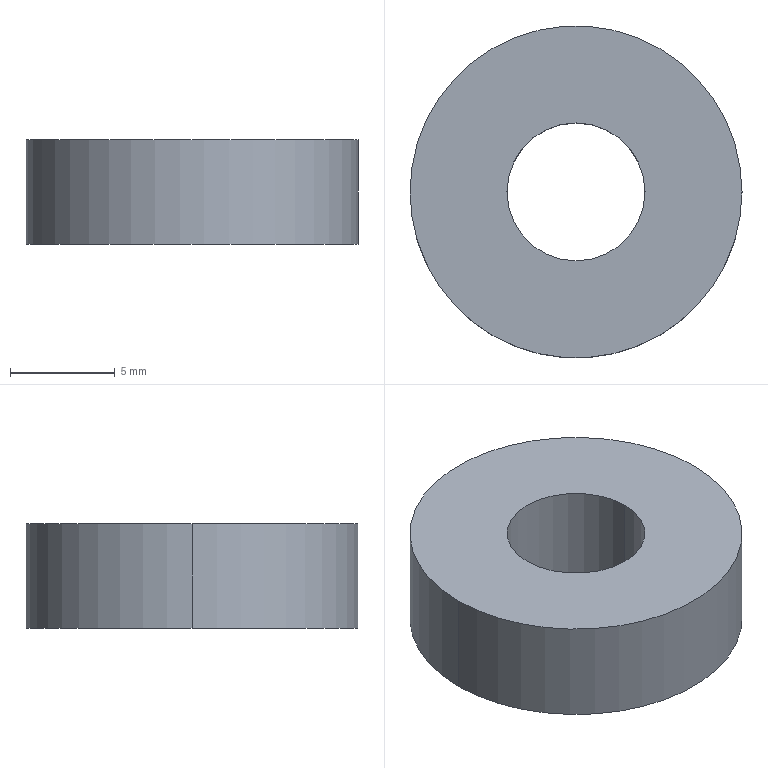Part | STEP file | 1_id922_x_t | 1 solid | 6 faces | box 15.876 x 15.876 x 5 mm | volume 818.728 mm3 | cylinder 4 | plane 2 | commonest cylinder face diameters 6.6 x2 15.876 x2
STEP:
#1=CARTESIAN_POINT('',(0.,0.,0.));
#2=DIRECTION('',(0.,0.,1.));
#3=DIRECTION('',(1.,0.,0.));
#4=AXIS2_PLACEMENT_3D('',#1,#2,#3);
#5=CARTESIAN_POINT('',(157.938,161.237,-7.7));
#6=VERTEX_POINT('',#5);
#7=CARTESIAN_POINT('',(142.062,161.237,-7.7));
#8=VERTEX_POINT('',#7);
#9=CARTESIAN_POINT('',(150.,161.237,-7.7));
#10=DIRECTION('',(0.,0.,1.));
#11=DIRECTION('',(1.,0.,0.));
#12=AXIS2_PLACEMENT_3D('',#9,#10,#11);
#13=CIRCLE('',#12,7.938);
#14=CARTESIAN_POINT('',(150.,161.237,-7.7));
#15=DIRECTION('',(0.,0.,-1.));
#16=DIRECTION('',(-1.,0.,0.));
#17=AXIS2_PLACEMENT_3D('',#14,#15,#16);
#18=PLANE('',#17);
#19=CARTESIAN_POINT('',(-7.938,0.));
#20=CARTESIAN_POINT('',(-7.938,13.749));
#21=CARTESIAN_POINT('',(3.969,6.875));
#22=CARTESIAN_POINT('',(15.876,0.));
#23=CARTESIAN_POINT('',(3.969,-6.875));
#24=CARTESIAN_POINT('',(-7.938,-13.749));
#25=CARTESIAN_POINT('',(-7.938,0.));
#26=(BOUNDED_CURVE()B_SPLINE_CURVE(2,(#19,#20,#21,#22,#23,#24,#25),.UNSPECIFIED.,.T.,.F.)B_SPLINE_CURVE_WITH_KNOTS((1,2,2,2,2,1),(-2.094,0.,2.094,4.189,6.283,8.378),.UNSPECIFIED.)CURVE()GEOMETRIC_REPRESENTATION_ITEM()RATIONAL_B_SPLINE_CURVE((1.,0.5,1.,0.5,1.,0.5,1.))REPRESENTATION_ITEM(''));
#27=(GEOMETRIC_REPRESENTATION_CONTEXT(2)PARAMETRIC_REPRESENTATION_CONTEXT()REPRESENTATION_CONTEXT('',''));
#28=DEFINITIONAL_REPRESENTATION('',(#26),#27);
#29=PCURVE('',#18,#28);
#30=CARTESIAN_POINT('',(150.,161.237,-7.7));
#31=DIRECTION('',(0.,0.,-1.));
#32=DIRECTION('',(-1.,0.,0.));
#33=AXIS2_PLACEMENT_3D('',#30,#31,#32);
#34=CYLINDRICAL_SURFACE('',#33,7.938);
#35=CARTESIAN_POINT('',(3.142,0.));
#36=DIRECTION('',(-1.,0.));
#37=VECTOR('',#36,1.);
#38=LINE('',#35,#37);
#39=(GEOMETRIC_REPRESENTATION_CONTEXT(2)PARAMETRIC_REPRESENTATION_CONTEXT()REPRESENTATION_CONTEXT('',''));
#40=DEFINITIONAL_REPRESENTATION('',(#38),#39);
#41=PCURVE('',#34,#40);
#42=SURFACE_CURVE('',#13,(#29,#41),.PCURVE_S1.);
#43=EDGE_CURVE('',#6,#8,#42,.T.);
#44=ORIENTED_EDGE('',*,*,#43,.T.);
#45=CARTESIAN_POINT('',(150.,161.237,-7.7));
#46=DIRECTION('',(0.,0.,1.));
#47=DIRECTION('',(-1.,0.,0.));
#48=AXIS2_PLACEMENT_3D('',#45,#46,#47);
#49=CIRCLE('',#48,7.938);
#50=CARTESIAN_POINT('',(7.938,0.));
#51=CARTESIAN_POINT('',(7.938,-13.749));
#52=CARTESIAN_POINT('',(-3.969,-6.875));
#53=CARTESIAN_POINT('',(-15.876,0.));
#54=CARTESIAN_POINT('',(-3.969,6.875));
#55=CARTESIAN_POINT('',(7.938,13.749));
#56=CARTESIAN_POINT('',(7.938,0.));
#57=(BOUNDED_CURVE()B_SPLINE_CURVE(2,(#50,#51,#52,#53,#54,#55,#56),.UNSPECIFIED.,.T.,.F.)B_SPLINE_CURVE_WITH_KNOTS((1,2,2,2,2,1),(-2.094,0.,2.094,4.189,6.283,8.378),.UNSPECIFIED.)CURVE()GEOMETRIC_REPRESENTATION_ITEM()RATIONAL_B_SPLINE_CURVE((1.,0.5,1.,0.5,1.,0.5,1.))REPRESENTATION_ITEM(''));
#58=(GEOMETRIC_REPRESENTATION_CONTEXT(2)PARAMETRIC_REPRESENTATION_CONTEXT()REPRESENTATION_CONTEXT('',''));
#59=DEFINITIONAL_REPRESENTATION('',(#57),#58);
#60=PCURVE('',#18,#59);
#61=CARTESIAN_POINT('',(150.,161.237,-7.7));
#62=DIRECTION('',(0.,0.,-1.));
#63=DIRECTION('',(-1.,0.,0.));
#64=AXIS2_PLACEMENT_3D('',#61,#62,#63);
#65=CYLINDRICAL_SURFACE('',#64,7.938);
#66=CARTESIAN_POINT('',(6.283,0.));
#67=DIRECTION('',(-1.,0.));
#68=VECTOR('',#67,1.);
#69=LINE('',#66,#68);
#70=(GEOMETRIC_REPRESENTATION_CONTEXT(2)PARAMETRIC_REPRESENTATION_CONTEXT()REPRESENTATION_CONTEXT('',''));
#71=DEFINITIONAL_REPRESENTATION('',(#69),#70);
#72=PCURVE('',#65,#71);
#73=SURFACE_CURVE('',#49,(#60,#72),.PCURVE_S1.);
#74=EDGE_CURVE('',#8,#6,#73,.T.);
#75=ORIENTED_EDGE('',*,*,#74,.T.);
#76=EDGE_LOOP('',(#44,#75));
#77=FACE_BOUND('',#76,.T.);
#78=CARTESIAN_POINT('',(146.7,161.237,-7.7));
#79=VERTEX_POINT('',#78);
#80=CARTESIAN_POINT('',(153.3,161.237,-7.7));
#81=VERTEX_POINT('',#80);
#82=CARTESIAN_POINT('',(150.,161.237,-7.7));
#83=DIRECTION('',(0.,0.,-1.));
#84=DIRECTION('',(-1.,0.,0.));
#85=AXIS2_PLACEMENT_3D('',#82,#83,#84);
#86=CIRCLE('',#85,3.3);
#87=CARTESIAN_POINT('',(0.,0.));
#88=DIRECTION('',(1.,0.));
#89=AXIS2_PLACEMENT_2D('',#87,#88);
#90=CIRCLE('',#89,3.3);
#91=(GEOMETRIC_REPRESENTATION_CONTEXT(2)PARAMETRIC_REPRESENTATION_CONTEXT()REPRESENTATION_CONTEXT('',''));
#92=DEFINITIONAL_REPRESENTATION('',(#90),#91);
#93=PCURVE('',#18,#92);
#94=CARTESIAN_POINT('',(150.,161.237,-35.7));
#95=DIRECTION('',(0.,0.,1.));
#96=DIRECTION('',(1.,0.,0.));
#97=AXIS2_PLACEMENT_3D('',#94,#95,#96);
#98=CYLINDRICAL_SURFACE('',#97,3.3);
#99=CARTESIAN_POINT('',(3.142,28.));
#100=DIRECTION('',(-1.,0.));
#101=VECTOR('',#100,1.);
#102=LINE('',#99,#101);
#103=(GEOMETRIC_REPRESENTATION_CONTEXT(2)PARAMETRIC_REPRESENTATION_CONTEXT()REPRESENTATION_CONTEXT('',''));
#104=DEFINITIONAL_REPRESENTATION('',(#102),#103);
#105=PCURVE('',#98,#104);
#106=SURFACE_CURVE('',#86,(#93,#105),.PCURVE_S1.);
#107=EDGE_CURVE('',#79,#81,#106,.T.);
#108=ORIENTED_EDGE('',*,*,#107,.T.);
#109=CARTESIAN_POINT('',(150.,161.237,-7.7));
#110=DIRECTION('',(0.,0.,-1.));
#111=DIRECTION('',(1.,0.,0.));
#112=AXIS2_PLACEMENT_3D('',#109,#110,#111);
#113=CIRCLE('',#112,3.3);
#114=CARTESIAN_POINT('',(0.,0.));
#115=DIRECTION('',(-1.,0.));
#116=AXIS2_PLACEMENT_2D('',#114,#115);
#117=CIRCLE('',#116,3.3);
#118=(GEOMETRIC_REPRESENTATION_CONTEXT(2)PARAMETRIC_REPRESENTATION_CONTEXT()REPRESENTATION_CONTEXT('',''));
#119=DEFINITIONAL_REPRESENTATION('',(#117),#118);
#120=PCURVE('',#18,#119);
#121=CARTESIAN_POINT('',(150.,161.237,-35.7));
#122=DIRECTION('',(0.,0.,1.));
#123=DIRECTION('',(1.,0.,0.));
#124=AXIS2_PLACEMENT_3D('',#121,#122,#123);
#125=CYLINDRICAL_SURFACE('',#124,3.3);
#126=CARTESIAN_POINT('',(6.283,28.));
#127=DIRECTION('',(-1.,0.));
#128=VECTOR('',#127,1.);
#129=LINE('',#126,#128);
#130=(GEOMETRIC_REPRESENTATION_CONTEXT(2)PARAMETRIC_REPRESENTATION_CONTEXT()REPRESENTATION_CONTEXT('',''));
#131=DEFINITIONAL_REPRESENTATION('',(#129),#130);
#132=PCURVE('',#125,#131);
#133=SURFACE_CURVE('',#113,(#120,#132),.PCURVE_S1.);
#134=EDGE_CURVE('',#81,#79,#133,.T.);
#135=ORIENTED_EDGE('',*,*,#134,.T.);
#136=EDGE_LOOP('',(#108,#135));
#137=FACE_BOUND('',#136,.T.);
#138=ADVANCED_FACE('',(#77,#137),#18,.F.);
#139=CARTESIAN_POINT('',(142.062,161.237,-12.7));
#140=VERTEX_POINT('',#139);
#141=CARTESIAN_POINT('',(142.062,161.237,-7.7));
#142=DIRECTION('',(0.,0.,-1.));
#143=VECTOR('',#142,1.);
#144=LINE('',#141,#143);
#145=CARTESIAN_POINT('',(6.283,0.));
#146=DIRECTION('',(0.,1.));
#147=VECTOR('',#146,1.);
#148=LINE('',#145,#147);
#149=(GEOMETRIC_REPRESENTATION_CONTEXT(2)PARAMETRIC_REPRESENTATION_CONTEXT()REPRESENTATION_CONTEXT('',''));
#150=DEFINITIONAL_REPRESENTATION('',(#148),#149);
#151=PCURVE('',#65,#150);
#152=CARTESIAN_POINT('',(0.,0.));
#153=DIRECTION('',(0.,1.));
#154=VECTOR('',#153,1.);
#155=LINE('',#152,#154);
#156=(GEOMETRIC_REPRESENTATION_CONTEXT(2)PARAMETRIC_REPRESENTATION_CONTEXT()REPRESENTATION_CONTEXT('',''));
#157=DEFINITIONAL_REPRESENTATION('',(#155),#156);
#158=PCURVE('',#34,#157);
#159=SURFACE_CURVE('',#144,(#151,#158),.PCURVE_S1.);
#160=EDGE_CURVE('',#8,#140,#159,.T.);
#161=ORIENTED_EDGE('',*,*,#160,.T.);
#162=CARTESIAN_POINT('',(157.938,161.237,-12.7));
#163=VERTEX_POINT('',#162);
#164=CARTESIAN_POINT('',(150.,161.237,-12.7));
#165=DIRECTION('',(0.,0.,-1.));
#166=DIRECTION('',(1.,0.,0.));
#167=AXIS2_PLACEMENT_3D('',#164,#165,#166);
#168=CIRCLE('',#167,7.938);
#169=CARTESIAN_POINT('',(3.142,5.));
#170=DIRECTION('',(1.,0.));
#171=VECTOR('',#170,1.);
#172=LINE('',#169,#171);
#173=(GEOMETRIC_REPRESENTATION_CONTEXT(2)PARAMETRIC_REPRESENTATION_CONTEXT()REPRESENTATION_CONTEXT('',''));
#174=DEFINITIONAL_REPRESENTATION('',(#172),#173);
#175=PCURVE('',#65,#174);
#176=CARTESIAN_POINT('',(150.,161.237,-12.7));
#177=DIRECTION('',(0.,0.,-1.));
#178=DIRECTION('',(-1.,0.,0.));
#179=AXIS2_PLACEMENT_3D('',#176,#177,#178);
#180=PLANE('',#179);
#181=CARTESIAN_POINT('',(0.,0.));
#182=DIRECTION('',(-1.,0.));
#183=AXIS2_PLACEMENT_2D('',#181,#182);
#184=CIRCLE('',#183,7.938);
#185=(GEOMETRIC_REPRESENTATION_CONTEXT(2)PARAMETRIC_REPRESENTATION_CONTEXT()REPRESENTATION_CONTEXT('',''));
#186=DEFINITIONAL_REPRESENTATION('',(#184),#185);
#187=PCURVE('',#180,#186);
#188=SURFACE_CURVE('',#168,(#175,#187),.PCURVE_S1.);
#189=EDGE_CURVE('',#163,#140,#188,.T.);
#190=ORIENTED_EDGE('',*,*,#189,.F.);
#191=CARTESIAN_POINT('',(157.938,161.237,-7.7));
#192=DIRECTION('',(0.,0.,1.));
#193=VECTOR('',#192,1.);
#194=LINE('',#191,#193);
#195=CARTESIAN_POINT('',(3.142,0.));
#196=DIRECTION('',(0.,-1.));
#197=VECTOR('',#196,1.);
#198=LINE('',#195,#197);
#199=(GEOMETRIC_REPRESENTATION_CONTEXT(2)PARAMETRIC_REPRESENTATION_CONTEXT()REPRESENTATION_CONTEXT('',''));
#200=DEFINITIONAL_REPRESENTATION('',(#198),#199);
#201=PCURVE('',#65,#200);
#202=CARTESIAN_POINT('',(3.142,0.));
#203=DIRECTION('',(0.,-1.));
#204=VECTOR('',#203,1.);
#205=LINE('',#202,#204);
#206=(GEOMETRIC_REPRESENTATION_CONTEXT(2)PARAMETRIC_REPRESENTATION_CONTEXT()REPRESENTATION_CONTEXT('',''));
#207=DEFINITIONAL_REPRESENTATION('',(#205),#206);
#208=PCURVE('',#34,#207);
#209=SURFACE_CURVE('',#194,(#201,#208),.PCURVE_S1.);
#210=EDGE_CURVE('',#163,#6,#209,.T.);
#211=ORIENTED_EDGE('',*,*,#210,.T.);
#212=ORIENTED_EDGE('',*,*,#74,.F.);
#213=EDGE_LOOP('',(#161,#190,#211,#212));
#214=FACE_BOUND('',#213,.T.);
#215=ADVANCED_FACE('',(#214),#65,.T.);
#216=ORIENTED_EDGE('',*,*,#210,.F.);
#217=CARTESIAN_POINT('',(150.,161.237,-12.7));
#218=DIRECTION('',(0.,0.,-1.));
#219=DIRECTION('',(-1.,0.,0.));
#220=AXIS2_PLACEMENT_3D('',#217,#218,#219);
#221=CIRCLE('',#220,7.938);
#222=CARTESIAN_POINT('',(0.,5.));
#223=DIRECTION('',(1.,0.));
#224=VECTOR('',#223,1.);
#225=LINE('',#222,#224);
#226=(GEOMETRIC_REPRESENTATION_CONTEXT(2)PARAMETRIC_REPRESENTATION_CONTEXT()REPRESENTATION_CONTEXT('',''));
#227=DEFINITIONAL_REPRESENTATION('',(#225),#226);
#228=PCURVE('',#34,#227);
#229=CARTESIAN_POINT('',(0.,0.));
#230=DIRECTION('',(1.,0.));
#231=AXIS2_PLACEMENT_2D('',#229,#230);
#232=CIRCLE('',#231,7.938);
#233=(GEOMETRIC_REPRESENTATION_CONTEXT(2)PARAMETRIC_REPRESENTATION_CONTEXT()REPRESENTATION_CONTEXT('',''));
#234=DEFINITIONAL_REPRESENTATION('',(#232),#233);
#235=PCURVE('',#180,#234);
#236=SURFACE_CURVE('',#221,(#228,#235),.PCURVE_S1.);
#237=EDGE_CURVE('',#140,#163,#236,.T.);
#238=ORIENTED_EDGE('',*,*,#237,.F.);
#239=ORIENTED_EDGE('',*,*,#160,.F.);
#240=ORIENTED_EDGE('',*,*,#43,.F.);
#241=EDGE_LOOP('',(#216,#238,#239,#240));
#242=FACE_BOUND('',#241,.T.);
#243=ADVANCED_FACE('',(#242),#34,.T.);
#244=ORIENTED_EDGE('',*,*,#189,.T.);
#245=ORIENTED_EDGE('',*,*,#237,.T.);
#246=EDGE_LOOP('',(#244,#245));
#247=FACE_BOUND('',#246,.T.);
#248=CARTESIAN_POINT('',(146.7,161.237,-12.7));
#249=VERTEX_POINT('',#248);
#250=CARTESIAN_POINT('',(153.3,161.237,-12.7));
#251=VERTEX_POINT('',#250);
#252=CARTESIAN_POINT('',(150.,161.237,-12.7));
#253=DIRECTION('',(0.,0.,1.));
#254=DIRECTION('',(-1.,0.,0.));
#255=AXIS2_PLACEMENT_3D('',#252,#253,#254);
#256=CIRCLE('',#255,3.3);
#257=CARTESIAN_POINT('',(3.3,0.));
#258=CARTESIAN_POINT('',(3.3,-5.716));
#259=CARTESIAN_POINT('',(-1.65,-2.858));
#260=CARTESIAN_POINT('',(-6.6,0.));
#261=CARTESIAN_POINT('',(-1.65,2.858));
#262=CARTESIAN_POINT('',(3.3,5.716));
#263=CARTESIAN_POINT('',(3.3,0.));
#264=(BOUNDED_CURVE()B_SPLINE_CURVE(2,(#257,#258,#259,#260,#261,#262,#263),.UNSPECIFIED.,.T.,.F.)B_SPLINE_CURVE_WITH_KNOTS((1,2,2,2,2,1),(-2.094,0.,2.094,4.189,6.283,8.378),.UNSPECIFIED.)CURVE()GEOMETRIC_REPRESENTATION_ITEM()RATIONAL_B_SPLINE_CURVE((1.,0.5,1.,0.5,1.,0.5,1.))REPRESENTATION_ITEM(''));
#265=(GEOMETRIC_REPRESENTATION_CONTEXT(2)PARAMETRIC_REPRESENTATION_CONTEXT()REPRESENTATION_CONTEXT('',''));
#266=DEFINITIONAL_REPRESENTATION('',(#264),#265);
#267=PCURVE('',#180,#266);
#268=CARTESIAN_POINT('',(3.142,23.));
#269=DIRECTION('',(1.,0.));
#270=VECTOR('',#269,1.);
#271=LINE('',#268,#270);
#272=(GEOMETRIC_REPRESENTATION_CONTEXT(2)PARAMETRIC_REPRESENTATION_CONTEXT()REPRESENTATION_CONTEXT('',''));
#273=DEFINITIONAL_REPRESENTATION('',(#271),#272);
#274=PCURVE('',#125,#273);
#275=SURFACE_CURVE('',#256,(#267,#274),.PCURVE_S1.);
#276=EDGE_CURVE('',#249,#251,#275,.T.);
#277=ORIENTED_EDGE('',*,*,#276,.T.);
#278=CARTESIAN_POINT('',(150.,161.237,-12.7));
#279=DIRECTION('',(0.,0.,1.));
#280=DIRECTION('',(1.,0.,0.));
#281=AXIS2_PLACEMENT_3D('',#278,#279,#280);
#282=CIRCLE('',#281,3.3);
#283=CARTESIAN_POINT('',(-3.3,0.));
#284=CARTESIAN_POINT('',(-3.3,5.716));
#285=CARTESIAN_POINT('',(1.65,2.858));
#286=CARTESIAN_POINT('',(6.6,0.));
#287=CARTESIAN_POINT('',(1.65,-2.858));
#288=CARTESIAN_POINT('',(-3.3,-5.716));
#289=CARTESIAN_POINT('',(-3.3,0.));
#290=(BOUNDED_CURVE()B_SPLINE_CURVE(2,(#283,#284,#285,#286,#287,#288,#289),.UNSPECIFIED.,.T.,.F.)B_SPLINE_CURVE_WITH_KNOTS((1,2,2,2,2,1),(-2.094,0.,2.094,4.189,6.283,8.378),.UNSPECIFIED.)CURVE()GEOMETRIC_REPRESENTATION_ITEM()RATIONAL_B_SPLINE_CURVE((1.,0.5,1.,0.5,1.,0.5,1.))REPRESENTATION_ITEM(''));
#291=(GEOMETRIC_REPRESENTATION_CONTEXT(2)PARAMETRIC_REPRESENTATION_CONTEXT()REPRESENTATION_CONTEXT('',''));
#292=DEFINITIONAL_REPRESENTATION('',(#290),#291);
#293=PCURVE('',#180,#292);
#294=CARTESIAN_POINT('',(0.,23.));
#295=DIRECTION('',(1.,0.));
#296=VECTOR('',#295,1.);
#297=LINE('',#294,#296);
#298=(GEOMETRIC_REPRESENTATION_CONTEXT(2)PARAMETRIC_REPRESENTATION_CONTEXT()REPRESENTATION_CONTEXT('',''));
#299=DEFINITIONAL_REPRESENTATION('',(#297),#298);
#300=PCURVE('',#98,#299);
#301=SURFACE_CURVE('',#282,(#293,#300),.PCURVE_S1.);
#302=EDGE_CURVE('',#251,#249,#301,.T.);
#303=ORIENTED_EDGE('',*,*,#302,.T.);
#304=EDGE_LOOP('',(#277,#303));
#305=FACE_BOUND('',#304,.T.);
#306=ADVANCED_FACE('',(#247,#305),#180,.T.);
#307=ORIENTED_EDGE('',*,*,#302,.T.);
#308=CARTESIAN_POINT('',(146.7,161.237,-12.7));
#309=DIRECTION('',(0.,0.,-1.));
#310=VECTOR('',#309,1.);
#311=LINE('',#308,#310);
#312=CARTESIAN_POINT('',(3.142,23.));
#313=DIRECTION('',(0.,-1.));
#314=VECTOR('',#313,1.);
#315=LINE('',#312,#314);
#316=(GEOMETRIC_REPRESENTATION_CONTEXT(2)PARAMETRIC_REPRESENTATION_CONTEXT()REPRESENTATION_CONTEXT('',''));
#317=DEFINITIONAL_REPRESENTATION('',(#315),#316);
#318=PCURVE('',#98,#317);
#319=CARTESIAN_POINT('',(3.142,23.));
#320=DIRECTION('',(0.,-1.));
#321=VECTOR('',#320,1.);
#322=LINE('',#319,#321);
#323=(GEOMETRIC_REPRESENTATION_CONTEXT(2)PARAMETRIC_REPRESENTATION_CONTEXT()REPRESENTATION_CONTEXT('',''));
#324=DEFINITIONAL_REPRESENTATION('',(#322),#323);
#325=PCURVE('',#125,#324);
#326=SURFACE_CURVE('',#311,(#318,#325),.PCURVE_S1.);
#327=EDGE_CURVE('',#79,#249,#326,.T.);
#328=ORIENTED_EDGE('',*,*,#327,.F.);
#329=ORIENTED_EDGE('',*,*,#107,.T.);
#330=CARTESIAN_POINT('',(153.3,161.237,-12.7));
#331=DIRECTION('',(0.,0.,1.));
#332=VECTOR('',#331,1.);
#333=LINE('',#330,#332);
#334=CARTESIAN_POINT('',(0.,23.));
#335=DIRECTION('',(0.,1.));
#336=VECTOR('',#335,1.);
#337=LINE('',#334,#336);
#338=(GEOMETRIC_REPRESENTATION_CONTEXT(2)PARAMETRIC_REPRESENTATION_CONTEXT()REPRESENTATION_CONTEXT('',''));
#339=DEFINITIONAL_REPRESENTATION('',(#337),#338);
#340=PCURVE('',#98,#339);
#341=CARTESIAN_POINT('',(6.283,23.));
#342=DIRECTION('',(0.,1.));
#343=VECTOR('',#342,1.);
#344=LINE('',#341,#343);
#345=(GEOMETRIC_REPRESENTATION_CONTEXT(2)PARAMETRIC_REPRESENTATION_CONTEXT()REPRESENTATION_CONTEXT('',''));
#346=DEFINITIONAL_REPRESENTATION('',(#344),#345);
#347=PCURVE('',#125,#346);
#348=SURFACE_CURVE('',#333,(#340,#347),.PCURVE_S1.);
#349=EDGE_CURVE('',#251,#81,#348,.T.);
#350=ORIENTED_EDGE('',*,*,#349,.F.);
#351=EDGE_LOOP('',(#307,#328,#329,#350));
#352=FACE_BOUND('',#351,.F.);
#353=ADVANCED_FACE('',(#352),#98,.F.);
#354=ORIENTED_EDGE('',*,*,#276,.T.);
#355=ORIENTED_EDGE('',*,*,#349,.T.);
#356=ORIENTED_EDGE('',*,*,#134,.T.);
#357=ORIENTED_EDGE('',*,*,#327,.T.);
#358=EDGE_LOOP('',(#354,#355,#356,#357));
#359=FACE_BOUND('',#358,.F.);
#360=ADVANCED_FACE('',(#359),#125,.F.);
#361=CLOSED_SHELL('',(#138,#215,#243,#306,#353,#360));
#362=MANIFOLD_SOLID_BREP('',#361);
#363=(LENGTH_UNIT()NAMED_UNIT(*)SI_UNIT(.MILLI.,.METRE.));
#364=UNCERTAINTY_MEASURE_WITH_UNIT(LENGTH_MEASURE(0.0000001),#363,'','');
#365=(NAMED_UNIT(*)PLANE_ANGLE_UNIT()SI_UNIT($,.RADIAN.));
#366=(NAMED_UNIT(*)SI_UNIT($,.STERADIAN.)SOLID_ANGLE_UNIT());
#367=(GEOMETRIC_REPRESENTATION_CONTEXT(3)GLOBAL_UNCERTAINTY_ASSIGNED_CONTEXT((#364))GLOBAL_UNIT_ASSIGNED_CONTEXT((#363,#365,#366))REPRESENTATION_CONTEXT('',''));
#368=ADVANCED_BREP_SHAPE_REPRESENTATION('',(#4,#362),#367);